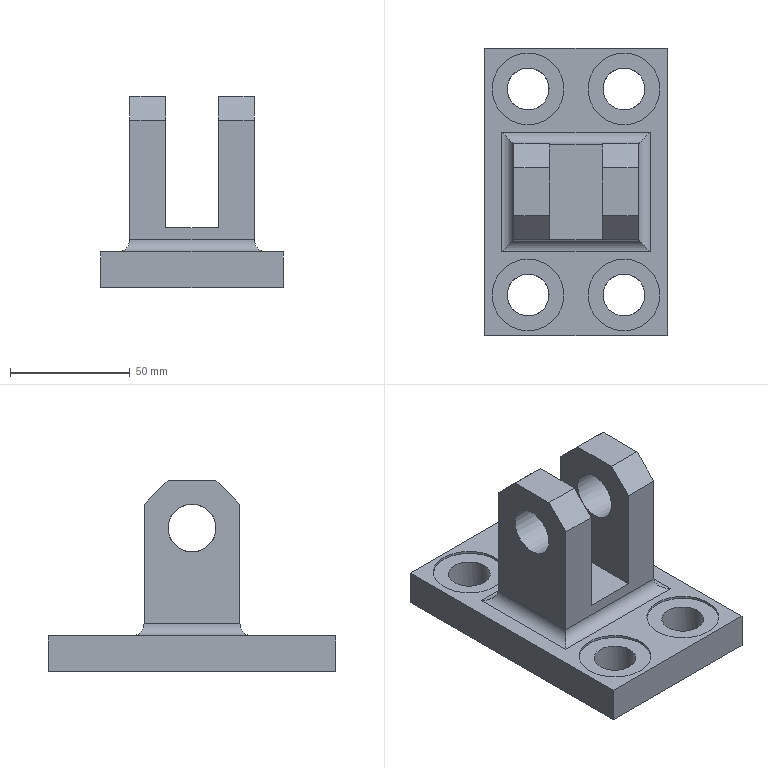Part | NX | features DATUM_CSYS 6, EXTRUDE 5, SKETCH 5, BLEND 1, CHAMFER 1 | 1 solid | 37 faces | box 76 x 120 x 80 mm | volume 195913 mm3 | plane 23 | cylinder 14 | commonest cylinder face diameters 10 x4 17.5 x4 30 x4 20 x2
STEP:
#1=CARTESIAN_POINT('',(20.,-34.25,0.));
#2=VERTEX_POINT('',#1);
#3=CARTESIAN_POINT('',(20.,-43.,0.));
#4=DIRECTION('',(0.,0.,1.));
#5=DIRECTION('',(0.,1.,0.));
#6=AXIS2_PLACEMENT_3D('',#3,#4,#5);
#7=CIRCLE('',#6,8.75);
#8=EDGE_CURVE('',#2,#2,#7,.T.);
#9=ORIENTED_EDGE('',*,*,#8,.F.);
#10=EDGE_LOOP('',(#9));
#11=FACE_BOUND('',#10,.T.);
#12=CARTESIAN_POINT('',(28.75,-43.,14.));
#13=VERTEX_POINT('',#12);
#14=CARTESIAN_POINT('',(20.,-43.,14.));
#15=DIRECTION('',(0.,0.,1.));
#16=DIRECTION('',(1.,0.,0.));
#17=AXIS2_PLACEMENT_3D('',#14,#15,#16);
#18=CIRCLE('',#17,8.75);
#19=EDGE_CURVE('',#13,#13,#18,.T.);
#20=ORIENTED_EDGE('',*,*,#19,.T.);
#21=EDGE_LOOP('',(#20));
#22=FACE_BOUND('',#21,.T.);
#23=CARTESIAN_POINT('',(20.,-43.,15.));
#24=DIRECTION('',(0.,0.,-1.));
#25=DIRECTION('',(-1.,0.,0.));
#26=AXIS2_PLACEMENT_3D('',#23,#24,#25);
#27=CYLINDRICAL_SURFACE('',#26,8.75);
#28=ADVANCED_FACE('',(#11,#22),#27,.F.);
#29=CARTESIAN_POINT('',(-20.,51.75,0.));
#30=VERTEX_POINT('',#29);
#31=CARTESIAN_POINT('',(-20.,43.,0.));
#32=DIRECTION('',(0.,0.,1.));
#33=DIRECTION('',(0.,1.,0.));
#34=AXIS2_PLACEMENT_3D('',#31,#32,#33);
#35=CIRCLE('',#34,8.75);
#36=EDGE_CURVE('',#30,#30,#35,.T.);
#37=ORIENTED_EDGE('',*,*,#36,.F.);
#38=EDGE_LOOP('',(#37));
#39=FACE_BOUND('',#38,.T.);
#40=CARTESIAN_POINT('',(-11.25,43.,14.));
#41=VERTEX_POINT('',#40);
#42=CARTESIAN_POINT('',(-20.,43.,14.));
#43=DIRECTION('',(0.,0.,1.));
#44=DIRECTION('',(1.,0.,0.));
#45=AXIS2_PLACEMENT_3D('',#42,#43,#44);
#46=CIRCLE('',#45,8.75);
#47=EDGE_CURVE('',#41,#41,#46,.T.);
#48=ORIENTED_EDGE('',*,*,#47,.T.);
#49=EDGE_LOOP('',(#48));
#50=FACE_BOUND('',#49,.T.);
#51=CARTESIAN_POINT('',(-20.,43.,15.));
#52=DIRECTION('',(0.,0.,-1.));
#53=DIRECTION('',(-1.,0.,0.));
#54=AXIS2_PLACEMENT_3D('',#51,#52,#53);
#55=CYLINDRICAL_SURFACE('',#54,8.75);
#56=ADVANCED_FACE('',(#39,#50),#55,.F.);
#57=CARTESIAN_POINT('',(-20.,-34.25,0.));
#58=VERTEX_POINT('',#57);
#59=CARTESIAN_POINT('',(-20.,-43.,0.));
#60=DIRECTION('',(0.,0.,1.));
#61=DIRECTION('',(0.,1.,0.));
#62=AXIS2_PLACEMENT_3D('',#59,#60,#61);
#63=CIRCLE('',#62,8.75);
#64=EDGE_CURVE('',#58,#58,#63,.T.);
#65=ORIENTED_EDGE('',*,*,#64,.F.);
#66=EDGE_LOOP('',(#65));
#67=FACE_BOUND('',#66,.T.);
#68=CARTESIAN_POINT('',(-11.25,-43.,14.));
#69=VERTEX_POINT('',#68);
#70=CARTESIAN_POINT('',(-20.,-43.,14.));
#71=DIRECTION('',(0.,0.,1.));
#72=DIRECTION('',(1.,0.,0.));
#73=AXIS2_PLACEMENT_3D('',#70,#71,#72);
#74=CIRCLE('',#73,8.75);
#75=EDGE_CURVE('',#69,#69,#74,.T.);
#76=ORIENTED_EDGE('',*,*,#75,.T.);
#77=EDGE_LOOP('',(#76));
#78=FACE_BOUND('',#77,.T.);
#79=CARTESIAN_POINT('',(-20.,-43.,15.));
#80=DIRECTION('',(0.,0.,-1.));
#81=DIRECTION('',(-1.,0.,0.));
#82=AXIS2_PLACEMENT_3D('',#79,#80,#81);
#83=CYLINDRICAL_SURFACE('',#82,8.75);
#84=ADVANCED_FACE('',(#67,#78),#83,.F.);
#85=CARTESIAN_POINT('',(20.,51.75,0.));
#86=VERTEX_POINT('',#85);
#87=CARTESIAN_POINT('',(20.,43.,0.));
#88=DIRECTION('',(0.,0.,1.));
#89=DIRECTION('',(0.,1.,0.));
#90=AXIS2_PLACEMENT_3D('',#87,#88,#89);
#91=CIRCLE('',#90,8.75);
#92=EDGE_CURVE('',#86,#86,#91,.T.);
#93=ORIENTED_EDGE('',*,*,#92,.F.);
#94=EDGE_LOOP('',(#93));
#95=FACE_BOUND('',#94,.T.);
#96=CARTESIAN_POINT('',(28.75,43.,14.));
#97=VERTEX_POINT('',#96);
#98=CARTESIAN_POINT('',(20.,43.,14.));
#99=DIRECTION('',(0.,0.,1.));
#100=DIRECTION('',(1.,0.,0.));
#101=AXIS2_PLACEMENT_3D('',#98,#99,#100);
#102=CIRCLE('',#101,8.75);
#103=EDGE_CURVE('',#97,#97,#102,.T.);
#104=ORIENTED_EDGE('',*,*,#103,.T.);
#105=EDGE_LOOP('',(#104));
#106=FACE_BOUND('',#105,.T.);
#107=CARTESIAN_POINT('',(20.,43.,15.));
#108=DIRECTION('',(0.,0.,-1.));
#109=DIRECTION('',(-1.,0.,0.));
#110=AXIS2_PLACEMENT_3D('',#107,#108,#109);
#111=CYLINDRICAL_SURFACE('',#110,8.75);
#112=ADVANCED_FACE('',(#95,#106),#111,.F.);
#113=CARTESIAN_POINT('',(-26.,-20.,70.));
#114=VERTEX_POINT('',#113);
#115=CARTESIAN_POINT('',(-26.,-20.,20.));
#116=VERTEX_POINT('',#115);
#117=CARTESIAN_POINT('',(-26.,-20.,80.));
#118=DIRECTION('',(0.,0.,-1.));
#119=VECTOR('',#118,1000.);
#120=LINE('',#117,#119);
#121=EDGE_CURVE('',#114,#116,#120,.T.);
#122=ORIENTED_EDGE('',*,*,#121,.T.);
#123=CARTESIAN_POINT('',(26.,-20.,20.));
#124=VERTEX_POINT('',#123);
#125=CARTESIAN_POINT('',(-26.,-20.,20.));
#126=DIRECTION('',(-1.,0.,0.));
#127=VECTOR('',#126,1000.);
#128=LINE('',#125,#127);
#129=EDGE_CURVE('',#116,#124,#128,.F.);
#130=ORIENTED_EDGE('',*,*,#129,.T.);
#131=CARTESIAN_POINT('',(26.,-20.,70.));
#132=VERTEX_POINT('',#131);
#133=CARTESIAN_POINT('',(26.,-20.,80.));
#134=DIRECTION('',(0.,0.,-1.));
#135=VECTOR('',#134,1000.);
#136=LINE('',#133,#135);
#137=EDGE_CURVE('',#132,#124,#136,.T.);
#138=ORIENTED_EDGE('',*,*,#137,.F.);
#139=CARTESIAN_POINT('',(11.,-20.,70.));
#140=VERTEX_POINT('',#139);
#141=CARTESIAN_POINT('',(11.,-20.,70.));
#142=DIRECTION('',(-1.,0.,0.));
#143=VECTOR('',#142,1000.);
#144=LINE('',#141,#143);
#145=EDGE_CURVE('',#132,#140,#144,.T.);
#146=ORIENTED_EDGE('',*,*,#145,.T.);
#147=CARTESIAN_POINT('',(11.,-20.,25.));
#148=VERTEX_POINT('',#147);
#149=CARTESIAN_POINT('',(11.,-20.,25.));
#150=DIRECTION('',(0.,0.,1.));
#151=VECTOR('',#150,1000.);
#152=LINE('',#149,#151);
#153=EDGE_CURVE('',#148,#140,#152,.T.);
#154=ORIENTED_EDGE('',*,*,#153,.F.);
#155=CARTESIAN_POINT('',(-11.,-20.,25.));
#156=VERTEX_POINT('',#155);
#157=CARTESIAN_POINT('',(-11.,-20.,25.));
#158=DIRECTION('',(1.,0.,0.));
#159=VECTOR('',#158,1000.);
#160=LINE('',#157,#159);
#161=EDGE_CURVE('',#156,#148,#160,.T.);
#162=ORIENTED_EDGE('',*,*,#161,.F.);
#163=CARTESIAN_POINT('',(-11.,-20.,70.));
#164=VERTEX_POINT('',#163);
#165=CARTESIAN_POINT('',(-11.,-20.,87.333));
#166=DIRECTION('',(0.,0.,-1.));
#167=VECTOR('',#166,1000.);
#168=LINE('',#165,#167);
#169=EDGE_CURVE('',#164,#156,#168,.T.);
#170=ORIENTED_EDGE('',*,*,#169,.F.);
#171=CARTESIAN_POINT('',(-26.,-20.,70.));
#172=DIRECTION('',(-1.,0.,0.));
#173=VECTOR('',#172,1000.);
#174=LINE('',#171,#173);
#175=EDGE_CURVE('',#164,#114,#174,.T.);
#176=ORIENTED_EDGE('',*,*,#175,.T.);
#177=EDGE_LOOP('',(#122,#130,#138,#146,#154,#162,#170,#176));
#178=FACE_BOUND('',#177,.T.);
#179=CARTESIAN_POINT('',(-26.,-20.,80.));
#180=DIRECTION('',(0.,1.,0.));
#181=DIRECTION('',(-1.,0.,0.));
#182=AXIS2_PLACEMENT_3D('',#179,#180,#181);
#183=PLANE('',#182);
#184=ADVANCED_FACE('',(#178),#183,.F.);
#185=CARTESIAN_POINT('',(-11.,10.,80.));
#186=VERTEX_POINT('',#185);
#187=CARTESIAN_POINT('',(-11.,-10.,80.));
#188=VERTEX_POINT('',#187);
#189=CARTESIAN_POINT('',(-11.,0.,80.));
#190=DIRECTION('',(0.,-1.,0.));
#191=VECTOR('',#190,1000.);
#192=LINE('',#189,#191);
#193=EDGE_CURVE('',#186,#188,#192,.T.);
#194=ORIENTED_EDGE('',*,*,#193,.F.);
#195=CARTESIAN_POINT('',(-26.,10.,80.));
#196=VERTEX_POINT('',#195);
#197=CARTESIAN_POINT('',(-26.,10.,80.));
#198=DIRECTION('',(-1.,0.,0.));
#199=VECTOR('',#198,1000.);
#200=LINE('',#197,#199);
#201=EDGE_CURVE('',#186,#196,#200,.T.);
#202=ORIENTED_EDGE('',*,*,#201,.T.);
#203=CARTESIAN_POINT('',(-26.,-10.,80.));
#204=VERTEX_POINT('',#203);
#205=CARTESIAN_POINT('',(-26.,20.,80.));
#206=DIRECTION('',(0.,-1.,0.));
#207=VECTOR('',#206,1000.);
#208=LINE('',#205,#207);
#209=EDGE_CURVE('',#196,#204,#208,.T.);
#210=ORIENTED_EDGE('',*,*,#209,.T.);
#211=CARTESIAN_POINT('',(-11.,-10.,80.));
#212=DIRECTION('',(1.,0.,0.));
#213=VECTOR('',#212,1000.);
#214=LINE('',#211,#213);
#215=EDGE_CURVE('',#204,#188,#214,.T.);
#216=ORIENTED_EDGE('',*,*,#215,.T.);
#217=EDGE_LOOP('',(#194,#202,#210,#216));
#218=FACE_BOUND('',#217,.T.);
#219=CARTESIAN_POINT('',(0.,0.,80.));
#220=DIRECTION('',(0.,0.,1.));
#221=DIRECTION('',(1.,0.,0.));
#222=AXIS2_PLACEMENT_3D('',#219,#220,#221);
#223=PLANE('',#222);
#224=ADVANCED_FACE('',(#218),#223,.T.);
#225=CARTESIAN_POINT('',(20.,-28.,15.));
#226=VERTEX_POINT('',#225);
#227=CARTESIAN_POINT('',(20.,-43.,15.));
#228=DIRECTION('',(0.,0.,1.));
#229=DIRECTION('',(0.,1.,0.));
#230=AXIS2_PLACEMENT_3D('',#227,#228,#229);
#231=CIRCLE('',#230,15.);
#232=EDGE_CURVE('',#226,#226,#231,.T.);
#233=ORIENTED_EDGE('',*,*,#232,.F.);
#234=EDGE_LOOP('',(#233));
#235=FACE_BOUND('',#234,.T.);
#236=CARTESIAN_POINT('',(-20.,58.,15.));
#237=VERTEX_POINT('',#236);
#238=CARTESIAN_POINT('',(-20.,43.,15.));
#239=DIRECTION('',(0.,0.,1.));
#240=DIRECTION('',(0.,1.,0.));
#241=AXIS2_PLACEMENT_3D('',#238,#239,#240);
#242=CIRCLE('',#241,15.);
#243=EDGE_CURVE('',#237,#237,#242,.T.);
#244=ORIENTED_EDGE('',*,*,#243,.F.);
#245=EDGE_LOOP('',(#244));
#246=FACE_BOUND('',#245,.T.);
#247=CARTESIAN_POINT('',(-20.,-28.,15.));
#248=VERTEX_POINT('',#247);
#249=CARTESIAN_POINT('',(-20.,-43.,15.));
#250=DIRECTION('',(0.,0.,1.));
#251=DIRECTION('',(0.,1.,0.));
#252=AXIS2_PLACEMENT_3D('',#249,#250,#251);
#253=CIRCLE('',#252,15.);
#254=EDGE_CURVE('',#248,#248,#253,.T.);
#255=ORIENTED_EDGE('',*,*,#254,.F.);
#256=EDGE_LOOP('',(#255));
#257=FACE_BOUND('',#256,.T.);
#258=CARTESIAN_POINT('',(20.,58.,15.));
#259=VERTEX_POINT('',#258);
#260=CARTESIAN_POINT('',(20.,43.,15.));
#261=DIRECTION('',(0.,0.,1.));
#262=DIRECTION('',(0.,1.,0.));
#263=AXIS2_PLACEMENT_3D('',#260,#261,#262);
#264=CIRCLE('',#263,15.);
#265=EDGE_CURVE('',#259,#259,#264,.T.);
#266=ORIENTED_EDGE('',*,*,#265,.F.);
#267=EDGE_LOOP('',(#266));
#268=FACE_BOUND('',#267,.T.);
#269=CARTESIAN_POINT('',(31.,-25.,15.));
#270=VERTEX_POINT('',#269);
#271=CARTESIAN_POINT('',(-31.,-25.,15.));
#272=VERTEX_POINT('',#271);
#273=CARTESIAN_POINT('',(-20.,-25.,15.));
#274=DIRECTION('',(-1.,0.,0.));
#275=VECTOR('',#274,1000.);
#276=LINE('',#273,#275);
#277=EDGE_CURVE('',#270,#272,#276,.T.);
#278=ORIENTED_EDGE('',*,*,#277,.T.);
#279=CARTESIAN_POINT('',(-31.,25.,15.));
#280=VERTEX_POINT('',#279);
#281=CARTESIAN_POINT('',(-31.,-43.,15.));
#282=DIRECTION('',(0.,1.,0.));
#283=VECTOR('',#282,1000.);
#284=LINE('',#281,#283);
#285=EDGE_CURVE('',#272,#280,#284,.T.);
#286=ORIENTED_EDGE('',*,*,#285,.T.);
#287=CARTESIAN_POINT('',(31.,25.,15.));
#288=VERTEX_POINT('',#287);
#289=CARTESIAN_POINT('',(-20.,25.,15.));
#290=DIRECTION('',(1.,0.,0.));
#291=VECTOR('',#290,1000.);
#292=LINE('',#289,#291);
#293=EDGE_CURVE('',#280,#288,#292,.T.);
#294=ORIENTED_EDGE('',*,*,#293,.T.);
#295=CARTESIAN_POINT('',(31.,-43.,15.));
#296=DIRECTION('',(0.,-1.,0.));
#297=VECTOR('',#296,1000.);
#298=LINE('',#295,#297);
#299=EDGE_CURVE('',#288,#270,#298,.T.);
#300=ORIENTED_EDGE('',*,*,#299,.T.);
#301=EDGE_LOOP('',(#278,#286,#294,#300));
#302=FACE_BOUND('',#301,.T.);
#303=CARTESIAN_POINT('',(-38.,60.,15.));
#304=VERTEX_POINT('',#303);
#305=CARTESIAN_POINT('',(-38.,-60.,15.));
#306=VERTEX_POINT('',#305);
#307=CARTESIAN_POINT('',(-38.,60.,15.));
#308=DIRECTION('',(0.,-1.,0.));
#309=VECTOR('',#308,1000.);
#310=LINE('',#307,#309);
#311=EDGE_CURVE('',#304,#306,#310,.T.);
#312=ORIENTED_EDGE('',*,*,#311,.T.);
#313=CARTESIAN_POINT('',(38.,-60.,15.));
#314=VERTEX_POINT('',#313);
#315=CARTESIAN_POINT('',(-38.,-60.,15.));
#316=DIRECTION('',(1.,0.,0.));
#317=VECTOR('',#316,1000.);
#318=LINE('',#315,#317);
#319=EDGE_CURVE('',#306,#314,#318,.T.);
#320=ORIENTED_EDGE('',*,*,#319,.T.);
#321=CARTESIAN_POINT('',(38.,60.,15.));
#322=VERTEX_POINT('',#321);
#323=CARTESIAN_POINT('',(38.,-60.,15.));
#324=DIRECTION('',(0.,1.,0.));
#325=VECTOR('',#324,1000.);
#326=LINE('',#323,#325);
#327=EDGE_CURVE('',#314,#322,#326,.T.);
#328=ORIENTED_EDGE('',*,*,#327,.T.);
#329=CARTESIAN_POINT('',(38.,60.,15.));
#330=DIRECTION('',(-1.,0.,0.));
#331=VECTOR('',#330,1000.);
#332=LINE('',#329,#331);
#333=EDGE_CURVE('',#322,#304,#332,.T.);
#334=ORIENTED_EDGE('',*,*,#333,.T.);
#335=EDGE_LOOP('',(#312,#320,#328,#334));
#336=FACE_BOUND('',#335,.T.);
#337=CARTESIAN_POINT('',(-20.,-43.,15.));
#338=DIRECTION('',(0.,0.,1.));
#339=DIRECTION('',(1.,0.,0.));
#340=AXIS2_PLACEMENT_3D('',#337,#338,#339);
#341=PLANE('',#340);
#342=ADVANCED_FACE('',(#235,#246,#257,#268,#302,#336),#341,.T.);
#343=CARTESIAN_POINT('',(-38.,60.,0.));
#344=VERTEX_POINT('',#343);
#345=CARTESIAN_POINT('',(-38.,-60.,0.));
#346=VERTEX_POINT('',#345);
#347=CARTESIAN_POINT('',(-38.,60.,0.));
#348=DIRECTION('',(0.,-1.,0.));
#349=VECTOR('',#348,1000.);
#350=LINE('',#347,#349);
#351=EDGE_CURVE('',#344,#346,#350,.T.);
#352=ORIENTED_EDGE('',*,*,#351,.T.);
#353=CARTESIAN_POINT('',(-38.,-60.,15.));
#354=DIRECTION('',(0.,0.,-1.));
#355=VECTOR('',#354,1000.);
#356=LINE('',#353,#355);
#357=EDGE_CURVE('',#306,#346,#356,.T.);
#358=ORIENTED_EDGE('',*,*,#357,.F.);
#359=ORIENTED_EDGE('',*,*,#311,.F.);
#360=CARTESIAN_POINT('',(-38.,60.,15.));
#361=DIRECTION('',(0.,0.,-1.));
#362=VECTOR('',#361,1000.);
#363=LINE('',#360,#362);
#364=EDGE_CURVE('',#304,#344,#363,.T.);
#365=ORIENTED_EDGE('',*,*,#364,.T.);
#366=EDGE_LOOP('',(#352,#358,#359,#365));
#367=FACE_BOUND('',#366,.T.);
#368=CARTESIAN_POINT('',(-38.,60.,15.));
#369=DIRECTION('',(1.,0.,0.));
#370=DIRECTION('',(0.,0.,-1.));
#371=AXIS2_PLACEMENT_3D('',#368,#369,#370);
#372=PLANE('',#371);
#373=ADVANCED_FACE('',(#367),#372,.F.);
#374=CARTESIAN_POINT('',(38.,-60.,0.));
#375=VERTEX_POINT('',#374);
#376=CARTESIAN_POINT('',(-38.,-60.,0.));
#377=DIRECTION('',(1.,0.,0.));
#378=VECTOR('',#377,1000.);
#379=LINE('',#376,#378);
#380=EDGE_CURVE('',#346,#375,#379,.T.);
#381=ORIENTED_EDGE('',*,*,#380,.T.);
#382=CARTESIAN_POINT('',(38.,-60.,15.));
#383=DIRECTION('',(0.,0.,-1.));
#384=VECTOR('',#383,1000.);
#385=LINE('',#382,#384);
#386=EDGE_CURVE('',#314,#375,#385,.T.);
#387=ORIENTED_EDGE('',*,*,#386,.F.);
#388=ORIENTED_EDGE('',*,*,#319,.F.);
#389=ORIENTED_EDGE('',*,*,#357,.T.);
#390=EDGE_LOOP('',(#381,#387,#388,#389));
#391=FACE_BOUND('',#390,.T.);
#392=CARTESIAN_POINT('',(-38.,-60.,15.));
#393=DIRECTION('',(0.,1.,0.));
#394=DIRECTION('',(-1.,0.,0.));
#395=AXIS2_PLACEMENT_3D('',#392,#393,#394);
#396=PLANE('',#395);
#397=ADVANCED_FACE('',(#391),#396,.F.);
#398=CARTESIAN_POINT('',(38.,60.,0.));
#399=VERTEX_POINT('',#398);
#400=CARTESIAN_POINT('',(38.,-60.,0.));
#401=DIRECTION('',(0.,1.,0.));
#402=VECTOR('',#401,1000.);
#403=LINE('',#400,#402);
#404=EDGE_CURVE('',#375,#399,#403,.T.);
#405=ORIENTED_EDGE('',*,*,#404,.T.);
#406=CARTESIAN_POINT('',(38.,60.,15.));
#407=DIRECTION('',(0.,0.,-1.));
#408=VECTOR('',#407,1000.);
#409=LINE('',#406,#408);
#410=EDGE_CURVE('',#322,#399,#409,.T.);
#411=ORIENTED_EDGE('',*,*,#410,.F.);
#412=ORIENTED_EDGE('',*,*,#327,.F.);
#413=ORIENTED_EDGE('',*,*,#386,.T.);
#414=EDGE_LOOP('',(#405,#411,#412,#413));
#415=FACE_BOUND('',#414,.T.);
#416=CARTESIAN_POINT('',(38.,-60.,15.));
#417=DIRECTION('',(-1.,0.,0.));
#418=DIRECTION('',(0.,0.,1.));
#419=AXIS2_PLACEMENT_3D('',#416,#417,#418);
#420=PLANE('',#419);
#421=ADVANCED_FACE('',(#415),#420,.F.);
#422=CARTESIAN_POINT('',(38.,60.,0.));
#423=DIRECTION('',(-1.,0.,0.));
#424=VECTOR('',#423,1000.);
#425=LINE('',#422,#424);
#426=EDGE_CURVE('',#399,#344,#425,.T.);
#427=ORIENTED_EDGE('',*,*,#426,.T.);
#428=ORIENTED_EDGE('',*,*,#364,.F.);
#429=ORIENTED_EDGE('',*,*,#333,.F.);
#430=ORIENTED_EDGE('',*,*,#410,.T.);
#431=EDGE_LOOP('',(#427,#428,#429,#430));
#432=FACE_BOUND('',#431,.T.);
#433=CARTESIAN_POINT('',(38.,60.,15.));
#434=DIRECTION('',(0.,-1.,0.));
#435=DIRECTION('',(1.,0.,0.));
#436=AXIS2_PLACEMENT_3D('',#433,#434,#435);
#437=PLANE('',#436);
#438=ADVANCED_FACE('',(#432),#437,.F.);
#439=ORIENTED_EDGE('',*,*,#92,.T.);
#440=EDGE_LOOP('',(#439));
#441=FACE_BOUND('',#440,.T.);
#442=ORIENTED_EDGE('',*,*,#8,.T.);
#443=EDGE_LOOP('',(#442));
#444=FACE_BOUND('',#443,.T.);
#445=ORIENTED_EDGE('',*,*,#36,.T.);
#446=EDGE_LOOP('',(#445));
#447=FACE_BOUND('',#446,.T.);
#448=ORIENTED_EDGE('',*,*,#64,.T.);
#449=EDGE_LOOP('',(#448));
#450=FACE_BOUND('',#449,.T.);
#451=ORIENTED_EDGE('',*,*,#351,.F.);
#452=ORIENTED_EDGE('',*,*,#426,.F.);
#453=ORIENTED_EDGE('',*,*,#404,.F.);
#454=ORIENTED_EDGE('',*,*,#380,.F.);
#455=EDGE_LOOP('',(#451,#452,#453,#454));
#456=FACE_BOUND('',#455,.T.);
#457=CARTESIAN_POINT('',(-20.,-43.,0.));
#458=DIRECTION('',(0.,0.,1.));
#459=DIRECTION('',(1.,0.,0.));
#460=AXIS2_PLACEMENT_3D('',#457,#458,#459);
#461=PLANE('',#460);
#462=ADVANCED_FACE('',(#441,#444,#447,#450,#456),#461,.F.);
#463=CARTESIAN_POINT('',(-26.,10.,60.));
#464=VERTEX_POINT('',#463);
#465=CARTESIAN_POINT('',(-26.,0.,60.));
#466=DIRECTION('',(1.,0.,0.));
#467=DIRECTION('',(0.,1.,0.));
#468=AXIS2_PLACEMENT_3D('',#465,#466,#467);
#469=CIRCLE('',#468,10.);
#470=EDGE_CURVE('',#464,#464,#469,.T.);
#471=ORIENTED_EDGE('',*,*,#470,.T.);
#472=EDGE_LOOP('',(#471));
#473=FACE_BOUND('',#472,.T.);
#474=CARTESIAN_POINT('',(-26.,20.,70.));
#475=VERTEX_POINT('',#474);
#476=CARTESIAN_POINT('',(-26.,20.,20.));
#477=VERTEX_POINT('',#476);
#478=CARTESIAN_POINT('',(-26.,20.,80.));
#479=DIRECTION('',(0.,0.,-1.));
#480=VECTOR('',#479,1000.);
#481=LINE('',#478,#480);
#482=EDGE_CURVE('',#475,#477,#481,.T.);
#483=ORIENTED_EDGE('',*,*,#482,.T.);
#484=CARTESIAN_POINT('',(-26.,20.,20.));
#485=DIRECTION('',(0.,1.,0.));
#486=VECTOR('',#485,1000.);
#487=LINE('',#484,#486);
#488=EDGE_CURVE('',#477,#116,#487,.F.);
#489=ORIENTED_EDGE('',*,*,#488,.T.);
#490=ORIENTED_EDGE('',*,*,#121,.F.);
#491=CARTESIAN_POINT('',(-26.,-10.,80.));
#492=DIRECTION('',(0.,0.7071,0.7071));
#493=VECTOR('',#492,1000.);
#494=LINE('',#491,#493);
#495=EDGE_CURVE('',#114,#204,#494,.T.);
#496=ORIENTED_EDGE('',*,*,#495,.T.);
#497=ORIENTED_EDGE('',*,*,#209,.F.);
#498=CARTESIAN_POINT('',(-26.,10.,80.));
#499=DIRECTION('',(0.,0.7071,-0.7071));
#500=VECTOR('',#499,1000.);
#501=LINE('',#498,#500);
#502=EDGE_CURVE('',#196,#475,#501,.T.);
#503=ORIENTED_EDGE('',*,*,#502,.T.);
#504=EDGE_LOOP('',(#483,#489,#490,#496,#497,#503));
#505=FACE_BOUND('',#504,.T.);
#506=CARTESIAN_POINT('',(-26.,20.,80.));
#507=DIRECTION('',(1.,0.,0.));
#508=DIRECTION('',(0.,1.,0.));
#509=AXIS2_PLACEMENT_3D('',#506,#507,#508);
#510=PLANE('',#509);
#511=ADVANCED_FACE('',(#473,#505),#510,.F.);
#512=CARTESIAN_POINT('',(26.,10.,60.));
#513=VERTEX_POINT('',#512);
#514=CARTESIAN_POINT('',(26.,0.,60.));
#515=DIRECTION('',(1.,0.,0.));
#516=DIRECTION('',(0.,1.,0.));
#517=AXIS2_PLACEMENT_3D('',#514,#515,#516);
#518=CIRCLE('',#517,10.);
#519=EDGE_CURVE('',#513,#513,#518,.T.);
#520=ORIENTED_EDGE('',*,*,#519,.F.);
#521=EDGE_LOOP('',(#520));
#522=FACE_BOUND('',#521,.T.);
#523=ORIENTED_EDGE('',*,*,#137,.T.);
#524=CARTESIAN_POINT('',(26.,20.,20.));
#525=VERTEX_POINT('',#524);
#526=CARTESIAN_POINT('',(26.,-20.,20.));
#527=DIRECTION('',(0.,-1.,0.));
#528=VECTOR('',#527,1000.);
#529=LINE('',#526,#528);
#530=EDGE_CURVE('',#124,#525,#529,.F.);
#531=ORIENTED_EDGE('',*,*,#530,.T.);
#532=CARTESIAN_POINT('',(26.,20.,70.));
#533=VERTEX_POINT('',#532);
#534=CARTESIAN_POINT('',(26.,20.,80.));
#535=DIRECTION('',(0.,0.,-1.));
#536=VECTOR('',#535,1000.);
#537=LINE('',#534,#536);
#538=EDGE_CURVE('',#533,#525,#537,.T.);
#539=ORIENTED_EDGE('',*,*,#538,.F.);
#540=CARTESIAN_POINT('',(26.,10.,80.));
#541=VERTEX_POINT('',#540);
#542=CARTESIAN_POINT('',(26.,10.,80.));
#543=DIRECTION('',(0.,-0.7071,0.7071));
#544=VECTOR('',#543,1000.);
#545=LINE('',#542,#544);
#546=EDGE_CURVE('',#533,#541,#545,.T.);
#547=ORIENTED_EDGE('',*,*,#546,.T.);
#548=CARTESIAN_POINT('',(26.,-10.,80.));
#549=VERTEX_POINT('',#548);
#550=CARTESIAN_POINT('',(26.,-20.,80.));
#551=DIRECTION('',(0.,1.,0.));
#552=VECTOR('',#551,1000.);
#553=LINE('',#550,#552);
#554=EDGE_CURVE('',#549,#541,#553,.T.);
#555=ORIENTED_EDGE('',*,*,#554,.F.);
#556=CARTESIAN_POINT('',(26.,-10.,80.));
#557=DIRECTION('',(0.,-0.7071,-0.7071));
#558=VECTOR('',#557,1000.);
#559=LINE('',#556,#558);
#560=EDGE_CURVE('',#549,#132,#559,.T.);
#561=ORIENTED_EDGE('',*,*,#560,.T.);
#562=EDGE_LOOP('',(#523,#531,#539,#547,#555,#561));
#563=FACE_BOUND('',#562,.T.);
#564=CARTESIAN_POINT('',(26.,-20.,80.));
#565=DIRECTION('',(-1.,0.,0.));
#566=DIRECTION('',(0.,0.,1.));
#567=AXIS2_PLACEMENT_3D('',#564,#565,#566);
#568=PLANE('',#567);
#569=ADVANCED_FACE('',(#522,#563),#568,.F.);
#570=ORIENTED_EDGE('',*,*,#538,.T.);
#571=CARTESIAN_POINT('',(26.,20.,20.));
#572=DIRECTION('',(1.,0.,0.));
#573=VECTOR('',#572,1000.);
#574=LINE('',#571,#573);
#575=EDGE_CURVE('',#525,#477,#574,.F.);
#576=ORIENTED_EDGE('',*,*,#575,.T.);
#577=ORIENTED_EDGE('',*,*,#482,.F.);
#578=CARTESIAN_POINT('',(-11.,20.,70.));
#579=VERTEX_POINT('',#578);
#580=CARTESIAN_POINT('',(-11.,20.,70.));
#581=DIRECTION('',(1.,0.,0.));
#582=VECTOR('',#581,1000.);
#583=LINE('',#580,#582);
#584=EDGE_CURVE('',#475,#579,#583,.T.);
#585=ORIENTED_EDGE('',*,*,#584,.T.);
#586=CARTESIAN_POINT('',(-11.,20.,25.));
#587=VERTEX_POINT('',#586);
#588=CARTESIAN_POINT('',(-11.,20.,80.));
#589=DIRECTION('',(0.,0.,-1.));
#590=VECTOR('',#589,1000.);
#591=LINE('',#588,#590);
#592=EDGE_CURVE('',#579,#587,#591,.T.);
#593=ORIENTED_EDGE('',*,*,#592,.T.);
#594=CARTESIAN_POINT('',(11.,20.,25.));
#595=VERTEX_POINT('',#594);
#596=CARTESIAN_POINT('',(26.,20.,25.));
#597=DIRECTION('',(1.,0.,0.));
#598=VECTOR('',#597,1000.);
#599=LINE('',#596,#598);
#600=EDGE_CURVE('',#587,#595,#599,.T.);
#601=ORIENTED_EDGE('',*,*,#600,.T.);
#602=CARTESIAN_POINT('',(11.,20.,70.));
#603=VERTEX_POINT('',#602);
#604=CARTESIAN_POINT('',(11.,20.,80.));
#605=DIRECTION('',(0.,0.,1.));
#606=VECTOR('',#605,1000.);
#607=LINE('',#604,#606);
#608=EDGE_CURVE('',#595,#603,#607,.T.);
#609=ORIENTED_EDGE('',*,*,#608,.T.);
#610=CARTESIAN_POINT('',(26.,20.,70.));
#611=DIRECTION('',(1.,0.,0.));
#612=VECTOR('',#611,1000.);
#613=LINE('',#610,#612);
#614=EDGE_CURVE('',#603,#533,#613,.T.);
#615=ORIENTED_EDGE('',*,*,#614,.T.);
#616=EDGE_LOOP('',(#570,#576,#577,#585,#593,#601,#609,#615));
#617=FACE_BOUND('',#616,.T.);
#618=CARTESIAN_POINT('',(26.,20.,80.));
#619=DIRECTION('',(0.,-1.,0.));
#620=DIRECTION('',(1.,0.,0.));
#621=AXIS2_PLACEMENT_3D('',#618,#619,#620);
#622=PLANE('',#621);
#623=ADVANCED_FACE('',(#617),#622,.F.);
#624=ORIENTED_EDGE('',*,*,#554,.T.);
#625=CARTESIAN_POINT('',(11.,10.,80.));
#626=VERTEX_POINT('',#625);
#627=CARTESIAN_POINT('',(11.,10.,80.));
#628=DIRECTION('',(-1.,0.,0.));
#629=VECTOR('',#628,1000.);
#630=LINE('',#627,#629);
#631=EDGE_CURVE('',#541,#626,#630,.T.);
#632=ORIENTED_EDGE('',*,*,#631,.T.);
#633=CARTESIAN_POINT('',(11.,-10.,80.));
#634=VERTEX_POINT('',#633);
#635=CARTESIAN_POINT('',(11.,0.,80.));
#636=DIRECTION('',(0.,1.,0.));
#637=VECTOR('',#636,1000.);
#638=LINE('',#635,#637);
#639=EDGE_CURVE('',#634,#626,#638,.T.);
#640=ORIENTED_EDGE('',*,*,#639,.F.);
#641=CARTESIAN_POINT('',(26.,-10.,80.));
#642=DIRECTION('',(1.,0.,0.));
#643=VECTOR('',#642,1000.);
#644=LINE('',#641,#643);
#645=EDGE_CURVE('',#634,#549,#644,.T.);
#646=ORIENTED_EDGE('',*,*,#645,.T.);
#647=EDGE_LOOP('',(#624,#632,#640,#646));
#648=FACE_BOUND('',#647,.T.);
#649=CARTESIAN_POINT('',(0.,0.,80.));
#650=DIRECTION('',(0.,0.,1.));
#651=DIRECTION('',(1.,0.,0.));
#652=AXIS2_PLACEMENT_3D('',#649,#650,#651);
#653=PLANE('',#652);
#654=ADVANCED_FACE('',(#648),#653,.T.);
#655=CARTESIAN_POINT('',(-11.,60.,25.));
#656=DIRECTION('',(0.,-1.,0.));
#657=VECTOR('',#656,1000.);
#658=LINE('',#655,#657);
#659=EDGE_CURVE('',#156,#587,#658,.F.);
#660=ORIENTED_EDGE('',*,*,#659,.F.);
#661=ORIENTED_EDGE('',*,*,#161,.T.);
#662=CARTESIAN_POINT('',(11.,60.,25.));
#663=DIRECTION('',(0.,-1.,0.));
#664=VECTOR('',#663,1000.);
#665=LINE('',#662,#664);
#666=EDGE_CURVE('',#148,#595,#665,.F.);
#667=ORIENTED_EDGE('',*,*,#666,.T.);
#668=ORIENTED_EDGE('',*,*,#600,.F.);
#669=EDGE_LOOP('',(#660,#661,#667,#668));
#670=FACE_BOUND('',#669,.T.);
#671=CARTESIAN_POINT('',(-11.,60.,25.));
#672=DIRECTION('',(0.,0.,-1.));
#673=DIRECTION('',(-1.,0.,0.));
#674=AXIS2_PLACEMENT_3D('',#671,#672,#673);
#675=PLANE('',#674);
#676=ADVANCED_FACE('',(#670),#675,.F.);
#677=CARTESIAN_POINT('',(-11.,0.,70.));
#678=VERTEX_POINT('',#677);
#679=CARTESIAN_POINT('',(-11.,0.,60.));
#680=DIRECTION('',(-1.,0.,0.));
#681=DIRECTION('',(0.,0.,1.));
#682=AXIS2_PLACEMENT_3D('',#679,#680,#681);
#683=CIRCLE('',#682,10.);
#684=EDGE_CURVE('',#678,#678,#683,.T.);
#685=ORIENTED_EDGE('',*,*,#684,.T.);
#686=EDGE_LOOP('',(#685));
#687=FACE_BOUND('',#686,.T.);
#688=ORIENTED_EDGE('',*,*,#592,.F.);
#689=CARTESIAN_POINT('',(-11.,10.,80.));
#690=DIRECTION('',(0.,-0.7071,0.7071));
#691=VECTOR('',#690,1000.);
#692=LINE('',#689,#691);
#693=EDGE_CURVE('',#579,#186,#692,.T.);
#694=ORIENTED_EDGE('',*,*,#693,.T.);
#695=ORIENTED_EDGE('',*,*,#193,.T.);
#696=CARTESIAN_POINT('',(-11.,-10.,80.));
#697=DIRECTION('',(0.,-0.7071,-0.7071));
#698=VECTOR('',#697,1000.);
#699=LINE('',#696,#698);
#700=EDGE_CURVE('',#188,#164,#699,.T.);
#701=ORIENTED_EDGE('',*,*,#700,.T.);
#702=ORIENTED_EDGE('',*,*,#169,.T.);
#703=ORIENTED_EDGE('',*,*,#659,.T.);
#704=EDGE_LOOP('',(#688,#694,#695,#701,#702,#703));
#705=FACE_BOUND('',#704,.T.);
#706=CARTESIAN_POINT('',(-11.,60.,87.333));
#707=DIRECTION('',(-1.,0.,0.));
#708=DIRECTION('',(0.,0.,1.));
#709=AXIS2_PLACEMENT_3D('',#706,#707,#708);
#710=PLANE('',#709);
#711=ADVANCED_FACE('',(#687,#705),#710,.F.);
#712=CARTESIAN_POINT('',(11.,0.,50.));
#713=VERTEX_POINT('',#712);
#714=CARTESIAN_POINT('',(11.,0.,60.));
#715=DIRECTION('',(1.,0.,0.));
#716=DIRECTION('',(0.,0.,-1.));
#717=AXIS2_PLACEMENT_3D('',#714,#715,#716);
#718=CIRCLE('',#717,10.);
#719=EDGE_CURVE('',#713,#713,#718,.T.);
#720=ORIENTED_EDGE('',*,*,#719,.T.);
#721=EDGE_LOOP('',(#720));
#722=FACE_BOUND('',#721,.T.);
#723=ORIENTED_EDGE('',*,*,#639,.T.);
#724=CARTESIAN_POINT('',(11.,10.,80.));
#725=DIRECTION('',(0.,0.7071,-0.7071));
#726=VECTOR('',#725,1000.);
#727=LINE('',#724,#726);
#728=EDGE_CURVE('',#626,#603,#727,.T.);
#729=ORIENTED_EDGE('',*,*,#728,.T.);
#730=ORIENTED_EDGE('',*,*,#608,.F.);
#731=ORIENTED_EDGE('',*,*,#666,.F.);
#732=ORIENTED_EDGE('',*,*,#153,.T.);
#733=CARTESIAN_POINT('',(11.,-10.,80.));
#734=DIRECTION('',(0.,0.7071,0.7071));
#735=VECTOR('',#734,1000.);
#736=LINE('',#733,#735);
#737=EDGE_CURVE('',#140,#634,#736,.T.);
#738=ORIENTED_EDGE('',*,*,#737,.T.);
#739=EDGE_LOOP('',(#723,#729,#730,#731,#732,#738));
#740=FACE_BOUND('',#739,.T.);
#741=CARTESIAN_POINT('',(11.,60.,25.));
#742=DIRECTION('',(1.,0.,0.));
#743=DIRECTION('',(0.,0.,-1.));
#744=AXIS2_PLACEMENT_3D('',#741,#742,#743);
#745=PLANE('',#744);
#746=ADVANCED_FACE('',(#722,#740),#745,.F.);
#747=ORIENTED_EDGE('',*,*,#519,.T.);
#748=EDGE_LOOP('',(#747));
#749=FACE_BOUND('',#748,.T.);
#750=ORIENTED_EDGE('',*,*,#719,.F.);
#751=EDGE_LOOP('',(#750));
#752=FACE_BOUND('',#751,.T.);
#753=CARTESIAN_POINT('',(-54.,0.,60.));
#754=DIRECTION('',(1.,0.,0.));
#755=DIRECTION('',(0.,0.,-1.));
#756=AXIS2_PLACEMENT_3D('',#753,#754,#755);
#757=CYLINDRICAL_SURFACE('',#756,10.);
#758=ADVANCED_FACE('',(#749,#752),#757,.F.);
#759=ORIENTED_EDGE('',*,*,#684,.F.);
#760=EDGE_LOOP('',(#759));
#761=FACE_BOUND('',#760,.T.);
#762=ORIENTED_EDGE('',*,*,#470,.F.);
#763=EDGE_LOOP('',(#762));
#764=FACE_BOUND('',#763,.T.);
#765=CARTESIAN_POINT('',(-54.,0.,60.));
#766=DIRECTION('',(1.,0.,0.));
#767=DIRECTION('',(0.,0.,-1.));
#768=AXIS2_PLACEMENT_3D('',#765,#766,#767);
#769=CYLINDRICAL_SURFACE('',#768,10.);
#770=ADVANCED_FACE('',(#761,#764),#769,.F.);
#771=ORIENTED_EDGE('',*,*,#546,.F.);
#772=ORIENTED_EDGE('',*,*,#614,.F.);
#773=ORIENTED_EDGE('',*,*,#728,.F.);
#774=ORIENTED_EDGE('',*,*,#631,.F.);
#775=EDGE_LOOP('',(#771,#772,#773,#774));
#776=FACE_BOUND('',#775,.T.);
#777=CARTESIAN_POINT('',(0.,10.,80.));
#778=DIRECTION('',(0.,0.7071,0.7071));
#779=DIRECTION('',(1.,0.,0.));
#780=AXIS2_PLACEMENT_3D('',#777,#778,#779);
#781=PLANE('',#780);
#782=ADVANCED_FACE('',(#776),#781,.T.);
#783=ORIENTED_EDGE('',*,*,#693,.F.);
#784=ORIENTED_EDGE('',*,*,#584,.F.);
#785=ORIENTED_EDGE('',*,*,#502,.F.);
#786=ORIENTED_EDGE('',*,*,#201,.F.);
#787=EDGE_LOOP('',(#783,#784,#785,#786));
#788=FACE_BOUND('',#787,.T.);
#789=CARTESIAN_POINT('',(0.,10.,80.));
#790=DIRECTION('',(0.,0.7071,0.7071));
#791=DIRECTION('',(1.,0.,0.));
#792=AXIS2_PLACEMENT_3D('',#789,#790,#791);
#793=PLANE('',#792);
#794=ADVANCED_FACE('',(#788),#793,.T.);
#795=ORIENTED_EDGE('',*,*,#737,.F.);
#796=ORIENTED_EDGE('',*,*,#145,.F.);
#797=ORIENTED_EDGE('',*,*,#560,.F.);
#798=ORIENTED_EDGE('',*,*,#645,.F.);
#799=EDGE_LOOP('',(#795,#796,#797,#798));
#800=FACE_BOUND('',#799,.T.);
#801=CARTESIAN_POINT('',(0.,-10.,80.));
#802=DIRECTION('',(0.,-0.7071,0.7071));
#803=DIRECTION('',(-1.,0.,0.));
#804=AXIS2_PLACEMENT_3D('',#801,#802,#803);
#805=PLANE('',#804);
#806=ADVANCED_FACE('',(#800),#805,.T.);
#807=ORIENTED_EDGE('',*,*,#495,.F.);
#808=ORIENTED_EDGE('',*,*,#175,.F.);
#809=ORIENTED_EDGE('',*,*,#700,.F.);
#810=ORIENTED_EDGE('',*,*,#215,.F.);
#811=EDGE_LOOP('',(#807,#808,#809,#810));
#812=FACE_BOUND('',#811,.T.);
#813=CARTESIAN_POINT('',(0.,-10.,80.));
#814=DIRECTION('',(0.,-0.7071,0.7071));
#815=DIRECTION('',(-1.,0.,0.));
#816=AXIS2_PLACEMENT_3D('',#813,#814,#815);
#817=PLANE('',#816);
#818=ADVANCED_FACE('',(#812),#817,.T.);
#819=CARTESIAN_POINT('',(31.,25.,20.));
#820=DIRECTION('',(0.7071,-0.7071,0.));
#821=DIRECTION('',(-0.7071,-0.7071,0.));
#822=AXIS2_PLACEMENT_3D('',#819,#820,#821);
#823=ELLIPSE('',#822,7.071,5.);
#824=EDGE_CURVE('',#525,#288,#823,.T.);
#825=ORIENTED_EDGE('',*,*,#824,.F.);
#826=ORIENTED_EDGE('',*,*,#530,.F.);
#827=CARTESIAN_POINT('',(31.,-25.,20.));
#828=DIRECTION('',(-0.7071,-0.7071,0.));
#829=DIRECTION('',(-0.7071,0.7071,0.));
#830=AXIS2_PLACEMENT_3D('',#827,#828,#829);
#831=ELLIPSE('',#830,7.071,5.);
#832=EDGE_CURVE('',#270,#124,#831,.F.);
#833=ORIENTED_EDGE('',*,*,#832,.F.);
#834=ORIENTED_EDGE('',*,*,#299,.F.);
#835=EDGE_LOOP('',(#825,#826,#833,#834));
#836=FACE_BOUND('',#835,.T.);
#837=CARTESIAN_POINT('',(31.,-43.,20.));
#838=DIRECTION('',(0.,-1.,0.));
#839=DIRECTION('',(0.,0.,-1.));
#840=AXIS2_PLACEMENT_3D('',#837,#838,#839);
#841=CYLINDRICAL_SURFACE('',#840,5.);
#842=ADVANCED_FACE('',(#836),#841,.F.);
#843=ORIENTED_EDGE('',*,*,#832,.T.);
#844=ORIENTED_EDGE('',*,*,#129,.F.);
#845=CARTESIAN_POINT('',(-31.,-25.,20.));
#846=DIRECTION('',(-0.7071,0.7071,0.));
#847=DIRECTION('',(-0.7071,-0.7071,0.));
#848=AXIS2_PLACEMENT_3D('',#845,#846,#847);
#849=ELLIPSE('',#848,7.071,5.);
#850=EDGE_CURVE('',#272,#116,#849,.F.);
#851=ORIENTED_EDGE('',*,*,#850,.F.);
#852=ORIENTED_EDGE('',*,*,#277,.F.);
#853=EDGE_LOOP('',(#843,#844,#851,#852));
#854=FACE_BOUND('',#853,.T.);
#855=CARTESIAN_POINT('',(-20.,-25.,20.));
#856=DIRECTION('',(-1.,0.,0.));
#857=DIRECTION('',(0.,-1.,0.));
#858=AXIS2_PLACEMENT_3D('',#855,#856,#857);
#859=CYLINDRICAL_SURFACE('',#858,5.);
#860=ADVANCED_FACE('',(#854),#859,.F.);
#861=ORIENTED_EDGE('',*,*,#824,.T.);
#862=ORIENTED_EDGE('',*,*,#293,.F.);
#863=CARTESIAN_POINT('',(-31.,25.,20.));
#864=DIRECTION('',(0.7071,0.7071,0.));
#865=DIRECTION('',(0.7071,-0.7071,0.));
#866=AXIS2_PLACEMENT_3D('',#863,#864,#865);
#867=ELLIPSE('',#866,7.071,5.);
#868=EDGE_CURVE('',#477,#280,#867,.T.);
#869=ORIENTED_EDGE('',*,*,#868,.F.);
#870=ORIENTED_EDGE('',*,*,#575,.F.);
#871=EDGE_LOOP('',(#861,#862,#869,#870));
#872=FACE_BOUND('',#871,.T.);
#873=CARTESIAN_POINT('',(-20.,25.,20.));
#874=DIRECTION('',(1.,0.,0.));
#875=DIRECTION('',(0.,1.,0.));
#876=AXIS2_PLACEMENT_3D('',#873,#874,#875);
#877=CYLINDRICAL_SURFACE('',#876,5.);
#878=ADVANCED_FACE('',(#872),#877,.F.);
#879=ORIENTED_EDGE('',*,*,#850,.T.);
#880=ORIENTED_EDGE('',*,*,#488,.F.);
#881=ORIENTED_EDGE('',*,*,#868,.T.);
#882=ORIENTED_EDGE('',*,*,#285,.F.);
#883=EDGE_LOOP('',(#879,#880,#881,#882));
#884=FACE_BOUND('',#883,.T.);
#885=CARTESIAN_POINT('',(-31.,-43.,20.));
#886=DIRECTION('',(0.,1.,0.));
#887=DIRECTION('',(-1.,0.,0.));
#888=AXIS2_PLACEMENT_3D('',#885,#886,#887);
#889=CYLINDRICAL_SURFACE('',#888,5.);
#890=ADVANCED_FACE('',(#884),#889,.F.);
#891=CARTESIAN_POINT('',(20.,58.,14.));
#892=VERTEX_POINT('',#891);
#893=CARTESIAN_POINT('',(20.,43.,14.));
#894=DIRECTION('',(0.,0.,1.));
#895=DIRECTION('',(0.,1.,0.));
#896=AXIS2_PLACEMENT_3D('',#893,#894,#895);
#897=CIRCLE('',#896,15.);
#898=EDGE_CURVE('',#892,#892,#897,.F.);
#899=ORIENTED_EDGE('',*,*,#898,.T.);
#900=EDGE_LOOP('',(#899));
#901=FACE_BOUND('',#900,.T.);
#902=ORIENTED_EDGE('',*,*,#265,.T.);
#903=EDGE_LOOP('',(#902));
#904=FACE_BOUND('',#903,.T.);
#905=CARTESIAN_POINT('',(20.,43.,14.));
#906=DIRECTION('',(0.,0.,1.));
#907=DIRECTION('',(1.,0.,0.));
#908=AXIS2_PLACEMENT_3D('',#905,#906,#907);
#909=CYLINDRICAL_SURFACE('',#908,15.);
#910=ADVANCED_FACE('',(#901,#904),#909,.F.);
#911=ORIENTED_EDGE('',*,*,#103,.F.);
#912=EDGE_LOOP('',(#911));
#913=FACE_BOUND('',#912,.T.);
#914=ORIENTED_EDGE('',*,*,#898,.F.);
#915=EDGE_LOOP('',(#914));
#916=FACE_BOUND('',#915,.T.);
#917=CARTESIAN_POINT('',(20.,43.,14.));
#918=DIRECTION('',(0.,0.,1.));
#919=DIRECTION('',(1.,0.,0.));
#920=AXIS2_PLACEMENT_3D('',#917,#918,#919);
#921=PLANE('',#920);
#922=ADVANCED_FACE('',(#913,#916),#921,.T.);
#923=CARTESIAN_POINT('',(-20.,-28.,14.));
#924=VERTEX_POINT('',#923);
#925=CARTESIAN_POINT('',(-20.,-43.,14.));
#926=DIRECTION('',(0.,0.,1.));
#927=DIRECTION('',(0.,1.,0.));
#928=AXIS2_PLACEMENT_3D('',#925,#926,#927);
#929=CIRCLE('',#928,15.);
#930=EDGE_CURVE('',#924,#924,#929,.F.);
#931=ORIENTED_EDGE('',*,*,#930,.T.);
#932=EDGE_LOOP('',(#931));
#933=FACE_BOUND('',#932,.T.);
#934=ORIENTED_EDGE('',*,*,#254,.T.);
#935=EDGE_LOOP('',(#934));
#936=FACE_BOUND('',#935,.T.);
#937=CARTESIAN_POINT('',(-20.,-43.,14.));
#938=DIRECTION('',(0.,0.,1.));
#939=DIRECTION('',(1.,0.,0.));
#940=AXIS2_PLACEMENT_3D('',#937,#938,#939);
#941=CYLINDRICAL_SURFACE('',#940,15.);
#942=ADVANCED_FACE('',(#933,#936),#941,.F.);
#943=ORIENTED_EDGE('',*,*,#75,.F.);
#944=EDGE_LOOP('',(#943));
#945=FACE_BOUND('',#944,.T.);
#946=ORIENTED_EDGE('',*,*,#930,.F.);
#947=EDGE_LOOP('',(#946));
#948=FACE_BOUND('',#947,.T.);
#949=CARTESIAN_POINT('',(-20.,-43.,14.));
#950=DIRECTION('',(0.,0.,1.));
#951=DIRECTION('',(1.,0.,0.));
#952=AXIS2_PLACEMENT_3D('',#949,#950,#951);
#953=PLANE('',#952);
#954=ADVANCED_FACE('',(#945,#948),#953,.T.);
#955=CARTESIAN_POINT('',(-20.,58.,14.));
#956=VERTEX_POINT('',#955);
#957=CARTESIAN_POINT('',(-20.,43.,14.));
#958=DIRECTION('',(0.,0.,1.));
#959=DIRECTION('',(0.,1.,0.));
#960=AXIS2_PLACEMENT_3D('',#957,#958,#959);
#961=CIRCLE('',#960,15.);
#962=EDGE_CURVE('',#956,#956,#961,.F.);
#963=ORIENTED_EDGE('',*,*,#962,.T.);
#964=EDGE_LOOP('',(#963));
#965=FACE_BOUND('',#964,.T.);
#966=ORIENTED_EDGE('',*,*,#243,.T.);
#967=EDGE_LOOP('',(#966));
#968=FACE_BOUND('',#967,.T.);
#969=CARTESIAN_POINT('',(-20.,43.,14.));
#970=DIRECTION('',(0.,0.,1.));
#971=DIRECTION('',(1.,0.,0.));
#972=AXIS2_PLACEMENT_3D('',#969,#970,#971);
#973=CYLINDRICAL_SURFACE('',#972,15.);
#974=ADVANCED_FACE('',(#965,#968),#973,.F.);
#975=ORIENTED_EDGE('',*,*,#47,.F.);
#976=EDGE_LOOP('',(#975));
#977=FACE_BOUND('',#976,.T.);
#978=ORIENTED_EDGE('',*,*,#962,.F.);
#979=EDGE_LOOP('',(#978));
#980=FACE_BOUND('',#979,.T.);
#981=CARTESIAN_POINT('',(-20.,43.,14.));
#982=DIRECTION('',(0.,0.,1.));
#983=DIRECTION('',(1.,0.,0.));
#984=AXIS2_PLACEMENT_3D('',#981,#982,#983);
#985=PLANE('',#984);
#986=ADVANCED_FACE('',(#977,#980),#985,.T.);
#987=CARTESIAN_POINT('',(20.,-28.,14.));
#988=VERTEX_POINT('',#987);
#989=CARTESIAN_POINT('',(20.,-43.,14.));
#990=DIRECTION('',(0.,0.,1.));
#991=DIRECTION('',(0.,1.,0.));
#992=AXIS2_PLACEMENT_3D('',#989,#990,#991);
#993=CIRCLE('',#992,15.);
#994=EDGE_CURVE('',#988,#988,#993,.F.);
#995=ORIENTED_EDGE('',*,*,#994,.T.);
#996=EDGE_LOOP('',(#995));
#997=FACE_BOUND('',#996,.T.);
#998=ORIENTED_EDGE('',*,*,#232,.T.);
#999=EDGE_LOOP('',(#998));
#1000=FACE_BOUND('',#999,.T.);
#1001=CARTESIAN_POINT('',(20.,-43.,14.));
#1002=DIRECTION('',(0.,0.,1.));
#1003=DIRECTION('',(1.,0.,0.));
#1004=AXIS2_PLACEMENT_3D('',#1001,#1002,#1003);
#1005=CYLINDRICAL_SURFACE('',#1004,15.);
#1006=ADVANCED_FACE('',(#997,#1000),#1005,.F.);
#1007=ORIENTED_EDGE('',*,*,#19,.F.);
#1008=EDGE_LOOP('',(#1007));
#1009=FACE_BOUND('',#1008,.T.);
#1010=ORIENTED_EDGE('',*,*,#994,.F.);
#1011=EDGE_LOOP('',(#1010));
#1012=FACE_BOUND('',#1011,.T.);
#1013=CARTESIAN_POINT('',(20.,-43.,14.));
#1014=DIRECTION('',(0.,0.,1.));
#1015=DIRECTION('',(1.,0.,0.));
#1016=AXIS2_PLACEMENT_3D('',#1013,#1014,#1015);
#1017=PLANE('',#1016);
#1018=ADVANCED_FACE('',(#1009,#1012),#1017,.T.);
#1019=CLOSED_SHELL('',(#28,#56,#84,#112,#184,#224,#342,#373,#397,#421,#438,#462,#511,#569,#623,#654,#676,#711,#746,#758,#770,#782,#794,#806,#818,#842,#860,#878,#890,#910,#922,#942,#954,#974,#986,#1006,#1018));
#1020=MANIFOLD_SOLID_BREP('',#1019);
#1021=(LENGTH_UNIT()NAMED_UNIT(*)SI_UNIT(.MILLI.,.METRE.));
#1022=UNCERTAINTY_MEASURE_WITH_UNIT(LENGTH_MEASURE(0.00001),#1021,'','');
#1023=(NAMED_UNIT(*)PLANE_ANGLE_UNIT()SI_UNIT($,.RADIAN.));
#1024=(NAMED_UNIT(*)SI_UNIT($,.STERADIAN.)SOLID_ANGLE_UNIT());
#1025=(GEOMETRIC_REPRESENTATION_CONTEXT(3)GLOBAL_UNCERTAINTY_ASSIGNED_CONTEXT((#1022))GLOBAL_UNIT_ASSIGNED_CONTEXT((#1021,#1023,#1024))REPRESENTATION_CONTEXT('',''));
#1026=ADVANCED_BREP_SHAPE_REPRESENTATION('',(#1020),#1025);